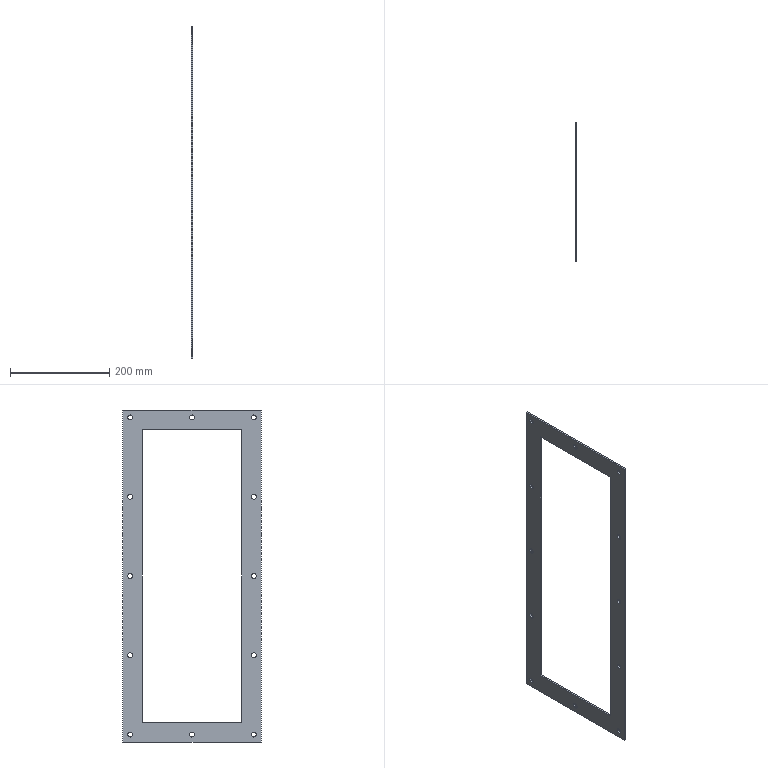Part | SolidWorks | features ExtruThin 1, HoleWzd 1, LPattern 1 | 1 solid | 34 faces | box 4 x 280 x 670 mm | volume 274630 mm3 | cylinder 24 | plane 10 | commonest cylinder face diameters 10 x24
STEP:
#1=CARTESIAN_POINT('',(0.,-125.,-315.));
#2=VERTEX_POINT('',#1);
#3=CARTESIAN_POINT('',(0.,-125.,-325.));
#4=VERTEX_POINT('',#3);
#5=CARTESIAN_POINT('',(0.,-125.,-320.));
#6=DIRECTION('',(1.,0.,0.));
#7=DIRECTION('',(0.,0.,-1.));
#8=AXIS2_PLACEMENT_3D('',#5,#6,#7);
#9=CIRCLE('',#8,5.);
#10=EDGE_CURVE('',#2,#4,#9,.T.);
#11=ORIENTED_EDGE('',*,*,#10,.F.);
#12=CARTESIAN_POINT('',(4.,-125.,-315.));
#13=VERTEX_POINT('',#12);
#14=CARTESIAN_POINT('',(4.,-125.,-315.));
#15=DIRECTION('',(1.,0.,0.));
#16=VECTOR('',#15,1000.);
#17=LINE('',#14,#16);
#18=EDGE_CURVE('',#2,#13,#17,.T.);
#19=ORIENTED_EDGE('',*,*,#18,.T.);
#20=CARTESIAN_POINT('',(4.,-125.,-325.));
#21=VERTEX_POINT('',#20);
#22=CARTESIAN_POINT('',(4.,-125.,-320.));
#23=DIRECTION('',(1.,0.,0.));
#24=DIRECTION('',(0.,0.,-1.));
#25=AXIS2_PLACEMENT_3D('',#22,#23,#24);
#26=CIRCLE('',#25,5.);
#27=EDGE_CURVE('',#13,#21,#26,.T.);
#28=ORIENTED_EDGE('',*,*,#27,.T.);
#29=CARTESIAN_POINT('',(4.,-125.,-325.));
#30=DIRECTION('',(1.,0.,0.));
#31=VECTOR('',#30,1000.);
#32=LINE('',#29,#31);
#33=EDGE_CURVE('',#4,#21,#32,.T.);
#34=ORIENTED_EDGE('',*,*,#33,.F.);
#35=EDGE_LOOP('',(#11,#19,#28,#34));
#36=FACE_OUTER_BOUND('',#35,.T.);
#37=CARTESIAN_POINT('',(4.,-125.,-320.));
#38=DIRECTION('',(1.,0.,0.));
#39=DIRECTION('',(0.,0.,-1.));
#40=AXIS2_PLACEMENT_3D('',#37,#38,#39);
#41=CYLINDRICAL_SURFACE('',#40,5.);
#42=ADVANCED_FACE('',(#36),#41,.F.);
#43=CARTESIAN_POINT('',(0.,0.,-315.));
#44=VERTEX_POINT('',#43);
#45=CARTESIAN_POINT('',(0.,0.,-325.));
#46=VERTEX_POINT('',#45);
#47=CARTESIAN_POINT('',(0.,0.,-320.));
#48=DIRECTION('',(1.,0.,0.));
#49=DIRECTION('',(0.,0.,-1.));
#50=AXIS2_PLACEMENT_3D('',#47,#48,#49);
#51=CIRCLE('',#50,5.);
#52=EDGE_CURVE('',#44,#46,#51,.T.);
#53=ORIENTED_EDGE('',*,*,#52,.F.);
#54=CARTESIAN_POINT('',(4.,0.,-315.));
#55=VERTEX_POINT('',#54);
#56=CARTESIAN_POINT('',(4.,0.,-315.));
#57=DIRECTION('',(1.,0.,0.));
#58=VECTOR('',#57,1000.);
#59=LINE('',#56,#58);
#60=EDGE_CURVE('',#44,#55,#59,.T.);
#61=ORIENTED_EDGE('',*,*,#60,.T.);
#62=CARTESIAN_POINT('',(4.,0.,-325.));
#63=VERTEX_POINT('',#62);
#64=CARTESIAN_POINT('',(4.,0.,-320.));
#65=DIRECTION('',(1.,0.,0.));
#66=DIRECTION('',(0.,0.,-1.));
#67=AXIS2_PLACEMENT_3D('',#64,#65,#66);
#68=CIRCLE('',#67,5.);
#69=EDGE_CURVE('',#55,#63,#68,.T.);
#70=ORIENTED_EDGE('',*,*,#69,.T.);
#71=CARTESIAN_POINT('',(4.,0.,-325.));
#72=DIRECTION('',(1.,0.,0.));
#73=VECTOR('',#72,1000.);
#74=LINE('',#71,#73);
#75=EDGE_CURVE('',#46,#63,#74,.T.);
#76=ORIENTED_EDGE('',*,*,#75,.F.);
#77=EDGE_LOOP('',(#53,#61,#70,#76));
#78=FACE_OUTER_BOUND('',#77,.T.);
#79=CARTESIAN_POINT('',(4.,0.,-320.));
#80=DIRECTION('',(1.,0.,0.));
#81=DIRECTION('',(0.,0.,-1.));
#82=AXIS2_PLACEMENT_3D('',#79,#80,#81);
#83=CYLINDRICAL_SURFACE('',#82,5.);
#84=ADVANCED_FACE('',(#78),#83,.F.);
#85=CARTESIAN_POINT('',(0.,125.,-315.));
#86=VERTEX_POINT('',#85);
#87=CARTESIAN_POINT('',(0.,125.,-325.));
#88=VERTEX_POINT('',#87);
#89=CARTESIAN_POINT('',(0.,125.,-320.));
#90=DIRECTION('',(1.,0.,0.));
#91=DIRECTION('',(0.,0.,-1.));
#92=AXIS2_PLACEMENT_3D('',#89,#90,#91);
#93=CIRCLE('',#92,5.);
#94=EDGE_CURVE('',#86,#88,#93,.T.);
#95=ORIENTED_EDGE('',*,*,#94,.F.);
#96=CARTESIAN_POINT('',(4.,125.,-315.));
#97=VERTEX_POINT('',#96);
#98=CARTESIAN_POINT('',(4.,125.,-315.));
#99=DIRECTION('',(1.,0.,0.));
#100=VECTOR('',#99,1000.);
#101=LINE('',#98,#100);
#102=EDGE_CURVE('',#86,#97,#101,.T.);
#103=ORIENTED_EDGE('',*,*,#102,.T.);
#104=CARTESIAN_POINT('',(4.,125.,-325.));
#105=VERTEX_POINT('',#104);
#106=CARTESIAN_POINT('',(4.,125.,-320.));
#107=DIRECTION('',(1.,0.,0.));
#108=DIRECTION('',(0.,0.,-1.));
#109=AXIS2_PLACEMENT_3D('',#106,#107,#108);
#110=CIRCLE('',#109,5.);
#111=EDGE_CURVE('',#97,#105,#110,.T.);
#112=ORIENTED_EDGE('',*,*,#111,.T.);
#113=CARTESIAN_POINT('',(4.,125.,-325.));
#114=DIRECTION('',(1.,0.,0.));
#115=VECTOR('',#114,1000.);
#116=LINE('',#113,#115);
#117=EDGE_CURVE('',#88,#105,#116,.T.);
#118=ORIENTED_EDGE('',*,*,#117,.F.);
#119=EDGE_LOOP('',(#95,#103,#112,#118));
#120=FACE_OUTER_BOUND('',#119,.T.);
#121=CARTESIAN_POINT('',(4.,125.,-320.));
#122=DIRECTION('',(1.,0.,0.));
#123=DIRECTION('',(0.,0.,-1.));
#124=AXIS2_PLACEMENT_3D('',#121,#122,#123);
#125=CYLINDRICAL_SURFACE('',#124,5.);
#126=ADVANCED_FACE('',(#120),#125,.F.);
#127=CARTESIAN_POINT('',(0.,-125.,-155.));
#128=VERTEX_POINT('',#127);
#129=CARTESIAN_POINT('',(0.,-125.,-165.));
#130=VERTEX_POINT('',#129);
#131=CARTESIAN_POINT('',(0.,-125.,-160.));
#132=DIRECTION('',(1.,0.,0.));
#133=DIRECTION('',(0.,0.,-1.));
#134=AXIS2_PLACEMENT_3D('',#131,#132,#133);
#135=CIRCLE('',#134,5.);
#136=EDGE_CURVE('',#128,#130,#135,.T.);
#137=ORIENTED_EDGE('',*,*,#136,.F.);
#138=CARTESIAN_POINT('',(4.,-125.,-155.));
#139=VERTEX_POINT('',#138);
#140=CARTESIAN_POINT('',(4.,-125.,-155.));
#141=DIRECTION('',(1.,0.,0.));
#142=VECTOR('',#141,1000.);
#143=LINE('',#140,#142);
#144=EDGE_CURVE('',#128,#139,#143,.T.);
#145=ORIENTED_EDGE('',*,*,#144,.T.);
#146=CARTESIAN_POINT('',(4.,-125.,-165.));
#147=VERTEX_POINT('',#146);
#148=CARTESIAN_POINT('',(4.,-125.,-160.));
#149=DIRECTION('',(1.,0.,0.));
#150=DIRECTION('',(0.,0.,-1.));
#151=AXIS2_PLACEMENT_3D('',#148,#149,#150);
#152=CIRCLE('',#151,5.);
#153=EDGE_CURVE('',#139,#147,#152,.T.);
#154=ORIENTED_EDGE('',*,*,#153,.T.);
#155=CARTESIAN_POINT('',(4.,-125.,-165.));
#156=DIRECTION('',(1.,0.,0.));
#157=VECTOR('',#156,1000.);
#158=LINE('',#155,#157);
#159=EDGE_CURVE('',#130,#147,#158,.T.);
#160=ORIENTED_EDGE('',*,*,#159,.F.);
#161=EDGE_LOOP('',(#137,#145,#154,#160));
#162=FACE_OUTER_BOUND('',#161,.T.);
#163=CARTESIAN_POINT('',(4.,-125.,-160.));
#164=DIRECTION('',(1.,0.,0.));
#165=DIRECTION('',(0.,0.,-1.));
#166=AXIS2_PLACEMENT_3D('',#163,#164,#165);
#167=CYLINDRICAL_SURFACE('',#166,5.);
#168=ADVANCED_FACE('',(#162),#167,.F.);
#169=CARTESIAN_POINT('',(0.,125.,-155.));
#170=VERTEX_POINT('',#169);
#171=CARTESIAN_POINT('',(0.,125.,-165.));
#172=VERTEX_POINT('',#171);
#173=CARTESIAN_POINT('',(0.,125.,-160.));
#174=DIRECTION('',(1.,0.,0.));
#175=DIRECTION('',(0.,0.,-1.));
#176=AXIS2_PLACEMENT_3D('',#173,#174,#175);
#177=CIRCLE('',#176,5.);
#178=EDGE_CURVE('',#170,#172,#177,.T.);
#179=ORIENTED_EDGE('',*,*,#178,.F.);
#180=CARTESIAN_POINT('',(4.,125.,-155.));
#181=VERTEX_POINT('',#180);
#182=CARTESIAN_POINT('',(4.,125.,-155.));
#183=DIRECTION('',(1.,0.,0.));
#184=VECTOR('',#183,1000.);
#185=LINE('',#182,#184);
#186=EDGE_CURVE('',#170,#181,#185,.T.);
#187=ORIENTED_EDGE('',*,*,#186,.T.);
#188=CARTESIAN_POINT('',(4.,125.,-165.));
#189=VERTEX_POINT('',#188);
#190=CARTESIAN_POINT('',(4.,125.,-160.));
#191=DIRECTION('',(1.,0.,0.));
#192=DIRECTION('',(0.,0.,-1.));
#193=AXIS2_PLACEMENT_3D('',#190,#191,#192);
#194=CIRCLE('',#193,5.);
#195=EDGE_CURVE('',#181,#189,#194,.T.);
#196=ORIENTED_EDGE('',*,*,#195,.T.);
#197=CARTESIAN_POINT('',(4.,125.,-165.));
#198=DIRECTION('',(1.,0.,0.));
#199=VECTOR('',#198,1000.);
#200=LINE('',#197,#199);
#201=EDGE_CURVE('',#172,#189,#200,.T.);
#202=ORIENTED_EDGE('',*,*,#201,.F.);
#203=EDGE_LOOP('',(#179,#187,#196,#202));
#204=FACE_OUTER_BOUND('',#203,.T.);
#205=CARTESIAN_POINT('',(4.,125.,-160.));
#206=DIRECTION('',(1.,0.,0.));
#207=DIRECTION('',(0.,0.,-1.));
#208=AXIS2_PLACEMENT_3D('',#205,#206,#207);
#209=CYLINDRICAL_SURFACE('',#208,5.);
#210=ADVANCED_FACE('',(#204),#209,.F.);
#211=CARTESIAN_POINT('',(0.,-125.,5.));
#212=VERTEX_POINT('',#211);
#213=CARTESIAN_POINT('',(0.,-125.,-5.));
#214=VERTEX_POINT('',#213);
#215=CARTESIAN_POINT('',(0.,-125.,0.));
#216=DIRECTION('',(1.,0.,0.));
#217=DIRECTION('',(0.,0.,-1.));
#218=AXIS2_PLACEMENT_3D('',#215,#216,#217);
#219=CIRCLE('',#218,5.);
#220=EDGE_CURVE('',#212,#214,#219,.T.);
#221=ORIENTED_EDGE('',*,*,#220,.F.);
#222=CARTESIAN_POINT('',(4.,-125.,5.));
#223=VERTEX_POINT('',#222);
#224=CARTESIAN_POINT('',(4.,-125.,5.));
#225=DIRECTION('',(1.,0.,0.));
#226=VECTOR('',#225,1000.);
#227=LINE('',#224,#226);
#228=EDGE_CURVE('',#212,#223,#227,.T.);
#229=ORIENTED_EDGE('',*,*,#228,.T.);
#230=CARTESIAN_POINT('',(4.,-125.,-5.));
#231=VERTEX_POINT('',#230);
#232=CARTESIAN_POINT('',(4.,-125.,0.));
#233=DIRECTION('',(1.,0.,0.));
#234=DIRECTION('',(0.,0.,-1.));
#235=AXIS2_PLACEMENT_3D('',#232,#233,#234);
#236=CIRCLE('',#235,5.);
#237=EDGE_CURVE('',#223,#231,#236,.T.);
#238=ORIENTED_EDGE('',*,*,#237,.T.);
#239=CARTESIAN_POINT('',(4.,-125.,-5.));
#240=DIRECTION('',(1.,0.,0.));
#241=VECTOR('',#240,1000.);
#242=LINE('',#239,#241);
#243=EDGE_CURVE('',#214,#231,#242,.T.);
#244=ORIENTED_EDGE('',*,*,#243,.F.);
#245=EDGE_LOOP('',(#221,#229,#238,#244));
#246=FACE_OUTER_BOUND('',#245,.T.);
#247=CARTESIAN_POINT('',(4.,-125.,0.));
#248=DIRECTION('',(1.,0.,0.));
#249=DIRECTION('',(0.,0.,-1.));
#250=AXIS2_PLACEMENT_3D('',#247,#248,#249);
#251=CYLINDRICAL_SURFACE('',#250,5.);
#252=ADVANCED_FACE('',(#246),#251,.F.);
#253=CARTESIAN_POINT('',(0.,125.,5.));
#254=VERTEX_POINT('',#253);
#255=CARTESIAN_POINT('',(0.,125.,-5.));
#256=VERTEX_POINT('',#255);
#257=CARTESIAN_POINT('',(0.,125.,0.));
#258=DIRECTION('',(1.,0.,0.));
#259=DIRECTION('',(0.,0.,-1.));
#260=AXIS2_PLACEMENT_3D('',#257,#258,#259);
#261=CIRCLE('',#260,5.);
#262=EDGE_CURVE('',#254,#256,#261,.T.);
#263=ORIENTED_EDGE('',*,*,#262,.F.);
#264=CARTESIAN_POINT('',(4.,125.,5.));
#265=VERTEX_POINT('',#264);
#266=CARTESIAN_POINT('',(4.,125.,5.));
#267=DIRECTION('',(1.,0.,0.));
#268=VECTOR('',#267,1000.);
#269=LINE('',#266,#268);
#270=EDGE_CURVE('',#254,#265,#269,.T.);
#271=ORIENTED_EDGE('',*,*,#270,.T.);
#272=CARTESIAN_POINT('',(4.,125.,-5.));
#273=VERTEX_POINT('',#272);
#274=CARTESIAN_POINT('',(4.,125.,0.));
#275=DIRECTION('',(1.,0.,0.));
#276=DIRECTION('',(0.,0.,-1.));
#277=AXIS2_PLACEMENT_3D('',#274,#275,#276);
#278=CIRCLE('',#277,5.);
#279=EDGE_CURVE('',#265,#273,#278,.T.);
#280=ORIENTED_EDGE('',*,*,#279,.T.);
#281=CARTESIAN_POINT('',(4.,125.,-5.));
#282=DIRECTION('',(1.,0.,0.));
#283=VECTOR('',#282,1000.);
#284=LINE('',#281,#283);
#285=EDGE_CURVE('',#256,#273,#284,.T.);
#286=ORIENTED_EDGE('',*,*,#285,.F.);
#287=EDGE_LOOP('',(#263,#271,#280,#286));
#288=FACE_OUTER_BOUND('',#287,.T.);
#289=CARTESIAN_POINT('',(4.,125.,0.));
#290=DIRECTION('',(1.,0.,0.));
#291=DIRECTION('',(0.,0.,-1.));
#292=AXIS2_PLACEMENT_3D('',#289,#290,#291);
#293=CYLINDRICAL_SURFACE('',#292,5.);
#294=ADVANCED_FACE('',(#288),#293,.F.);
#295=CARTESIAN_POINT('',(0.,-125.,165.));
#296=VERTEX_POINT('',#295);
#297=CARTESIAN_POINT('',(0.,-125.,155.));
#298=VERTEX_POINT('',#297);
#299=CARTESIAN_POINT('',(0.,-125.,160.));
#300=DIRECTION('',(1.,0.,0.));
#301=DIRECTION('',(0.,0.,-1.));
#302=AXIS2_PLACEMENT_3D('',#299,#300,#301);
#303=CIRCLE('',#302,5.);
#304=EDGE_CURVE('',#296,#298,#303,.T.);
#305=ORIENTED_EDGE('',*,*,#304,.F.);
#306=CARTESIAN_POINT('',(4.,-125.,165.));
#307=VERTEX_POINT('',#306);
#308=CARTESIAN_POINT('',(4.,-125.,165.));
#309=DIRECTION('',(1.,0.,0.));
#310=VECTOR('',#309,1000.);
#311=LINE('',#308,#310);
#312=EDGE_CURVE('',#296,#307,#311,.T.);
#313=ORIENTED_EDGE('',*,*,#312,.T.);
#314=CARTESIAN_POINT('',(4.,-125.,155.));
#315=VERTEX_POINT('',#314);
#316=CARTESIAN_POINT('',(4.,-125.,160.));
#317=DIRECTION('',(1.,0.,0.));
#318=DIRECTION('',(0.,0.,-1.));
#319=AXIS2_PLACEMENT_3D('',#316,#317,#318);
#320=CIRCLE('',#319,5.);
#321=EDGE_CURVE('',#307,#315,#320,.T.);
#322=ORIENTED_EDGE('',*,*,#321,.T.);
#323=CARTESIAN_POINT('',(4.,-125.,155.));
#324=DIRECTION('',(1.,0.,0.));
#325=VECTOR('',#324,1000.);
#326=LINE('',#323,#325);
#327=EDGE_CURVE('',#298,#315,#326,.T.);
#328=ORIENTED_EDGE('',*,*,#327,.F.);
#329=EDGE_LOOP('',(#305,#313,#322,#328));
#330=FACE_OUTER_BOUND('',#329,.T.);
#331=CARTESIAN_POINT('',(4.,-125.,160.));
#332=DIRECTION('',(1.,0.,0.));
#333=DIRECTION('',(0.,0.,-1.));
#334=AXIS2_PLACEMENT_3D('',#331,#332,#333);
#335=CYLINDRICAL_SURFACE('',#334,5.);
#336=ADVANCED_FACE('',(#330),#335,.F.);
#337=CARTESIAN_POINT('',(0.,125.,165.));
#338=VERTEX_POINT('',#337);
#339=CARTESIAN_POINT('',(0.,125.,155.));
#340=VERTEX_POINT('',#339);
#341=CARTESIAN_POINT('',(0.,125.,160.));
#342=DIRECTION('',(1.,0.,0.));
#343=DIRECTION('',(0.,0.,-1.));
#344=AXIS2_PLACEMENT_3D('',#341,#342,#343);
#345=CIRCLE('',#344,5.);
#346=EDGE_CURVE('',#338,#340,#345,.T.);
#347=ORIENTED_EDGE('',*,*,#346,.F.);
#348=CARTESIAN_POINT('',(4.,125.,165.));
#349=VERTEX_POINT('',#348);
#350=CARTESIAN_POINT('',(4.,125.,165.));
#351=DIRECTION('',(1.,0.,0.));
#352=VECTOR('',#351,1000.);
#353=LINE('',#350,#352);
#354=EDGE_CURVE('',#338,#349,#353,.T.);
#355=ORIENTED_EDGE('',*,*,#354,.T.);
#356=CARTESIAN_POINT('',(4.,125.,155.));
#357=VERTEX_POINT('',#356);
#358=CARTESIAN_POINT('',(4.,125.,160.));
#359=DIRECTION('',(1.,0.,0.));
#360=DIRECTION('',(0.,0.,-1.));
#361=AXIS2_PLACEMENT_3D('',#358,#359,#360);
#362=CIRCLE('',#361,5.);
#363=EDGE_CURVE('',#349,#357,#362,.T.);
#364=ORIENTED_EDGE('',*,*,#363,.T.);
#365=CARTESIAN_POINT('',(4.,125.,155.));
#366=DIRECTION('',(1.,0.,0.));
#367=VECTOR('',#366,1000.);
#368=LINE('',#365,#367);
#369=EDGE_CURVE('',#340,#357,#368,.T.);
#370=ORIENTED_EDGE('',*,*,#369,.F.);
#371=EDGE_LOOP('',(#347,#355,#364,#370));
#372=FACE_OUTER_BOUND('',#371,.T.);
#373=CARTESIAN_POINT('',(4.,125.,160.));
#374=DIRECTION('',(1.,0.,0.));
#375=DIRECTION('',(0.,0.,-1.));
#376=AXIS2_PLACEMENT_3D('',#373,#374,#375);
#377=CYLINDRICAL_SURFACE('',#376,5.);
#378=ADVANCED_FACE('',(#372),#377,.F.);
#379=CARTESIAN_POINT('',(0.,-125.,325.));
#380=VERTEX_POINT('',#379);
#381=CARTESIAN_POINT('',(0.,-125.,315.));
#382=VERTEX_POINT('',#381);
#383=CARTESIAN_POINT('',(0.,-125.,320.));
#384=DIRECTION('',(1.,0.,0.));
#385=DIRECTION('',(0.,0.,-1.));
#386=AXIS2_PLACEMENT_3D('',#383,#384,#385);
#387=CIRCLE('',#386,5.);
#388=EDGE_CURVE('',#380,#382,#387,.T.);
#389=ORIENTED_EDGE('',*,*,#388,.F.);
#390=CARTESIAN_POINT('',(4.,-125.,325.));
#391=VERTEX_POINT('',#390);
#392=CARTESIAN_POINT('',(4.,-125.,325.));
#393=DIRECTION('',(1.,0.,0.));
#394=VECTOR('',#393,1000.);
#395=LINE('',#392,#394);
#396=EDGE_CURVE('',#380,#391,#395,.T.);
#397=ORIENTED_EDGE('',*,*,#396,.T.);
#398=CARTESIAN_POINT('',(4.,-125.,315.));
#399=VERTEX_POINT('',#398);
#400=CARTESIAN_POINT('',(4.,-125.,320.));
#401=DIRECTION('',(1.,0.,0.));
#402=DIRECTION('',(0.,0.,-1.));
#403=AXIS2_PLACEMENT_3D('',#400,#401,#402);
#404=CIRCLE('',#403,5.);
#405=EDGE_CURVE('',#391,#399,#404,.T.);
#406=ORIENTED_EDGE('',*,*,#405,.T.);
#407=CARTESIAN_POINT('',(4.,-125.,315.));
#408=DIRECTION('',(1.,0.,0.));
#409=VECTOR('',#408,1000.);
#410=LINE('',#407,#409);
#411=EDGE_CURVE('',#382,#399,#410,.T.);
#412=ORIENTED_EDGE('',*,*,#411,.F.);
#413=EDGE_LOOP('',(#389,#397,#406,#412));
#414=FACE_OUTER_BOUND('',#413,.T.);
#415=CARTESIAN_POINT('',(4.,-125.,320.));
#416=DIRECTION('',(1.,0.,0.));
#417=DIRECTION('',(0.,0.,-1.));
#418=AXIS2_PLACEMENT_3D('',#415,#416,#417);
#419=CYLINDRICAL_SURFACE('',#418,5.);
#420=ADVANCED_FACE('',(#414),#419,.F.);
#421=CARTESIAN_POINT('',(0.,0.,325.));
#422=VERTEX_POINT('',#421);
#423=CARTESIAN_POINT('',(0.,0.,315.));
#424=VERTEX_POINT('',#423);
#425=CARTESIAN_POINT('',(0.,0.,320.));
#426=DIRECTION('',(1.,0.,0.));
#427=DIRECTION('',(0.,0.,-1.));
#428=AXIS2_PLACEMENT_3D('',#425,#426,#427);
#429=CIRCLE('',#428,5.);
#430=EDGE_CURVE('',#422,#424,#429,.T.);
#431=ORIENTED_EDGE('',*,*,#430,.F.);
#432=CARTESIAN_POINT('',(4.,0.,325.));
#433=VERTEX_POINT('',#432);
#434=CARTESIAN_POINT('',(4.,0.,325.));
#435=DIRECTION('',(1.,0.,0.));
#436=VECTOR('',#435,1000.);
#437=LINE('',#434,#436);
#438=EDGE_CURVE('',#422,#433,#437,.T.);
#439=ORIENTED_EDGE('',*,*,#438,.T.);
#440=CARTESIAN_POINT('',(4.,0.,315.));
#441=VERTEX_POINT('',#440);
#442=CARTESIAN_POINT('',(4.,0.,320.));
#443=DIRECTION('',(1.,0.,0.));
#444=DIRECTION('',(0.,0.,-1.));
#445=AXIS2_PLACEMENT_3D('',#442,#443,#444);
#446=CIRCLE('',#445,5.);
#447=EDGE_CURVE('',#433,#441,#446,.T.);
#448=ORIENTED_EDGE('',*,*,#447,.T.);
#449=CARTESIAN_POINT('',(4.,0.,315.));
#450=DIRECTION('',(1.,0.,0.));
#451=VECTOR('',#450,1000.);
#452=LINE('',#449,#451);
#453=EDGE_CURVE('',#424,#441,#452,.T.);
#454=ORIENTED_EDGE('',*,*,#453,.F.);
#455=EDGE_LOOP('',(#431,#439,#448,#454));
#456=FACE_OUTER_BOUND('',#455,.T.);
#457=CARTESIAN_POINT('',(4.,0.,320.));
#458=DIRECTION('',(1.,0.,0.));
#459=DIRECTION('',(0.,0.,-1.));
#460=AXIS2_PLACEMENT_3D('',#457,#458,#459);
#461=CYLINDRICAL_SURFACE('',#460,5.);
#462=ADVANCED_FACE('',(#456),#461,.F.);
#463=CARTESIAN_POINT('',(0.,125.,325.));
#464=VERTEX_POINT('',#463);
#465=CARTESIAN_POINT('',(0.,125.,315.));
#466=VERTEX_POINT('',#465);
#467=CARTESIAN_POINT('',(0.,125.,320.));
#468=DIRECTION('',(1.,0.,0.));
#469=DIRECTION('',(0.,0.,-1.));
#470=AXIS2_PLACEMENT_3D('',#467,#468,#469);
#471=CIRCLE('',#470,5.);
#472=EDGE_CURVE('',#464,#466,#471,.T.);
#473=ORIENTED_EDGE('',*,*,#472,.F.);
#474=CARTESIAN_POINT('',(4.,125.,325.));
#475=VERTEX_POINT('',#474);
#476=CARTESIAN_POINT('',(4.,125.,325.));
#477=DIRECTION('',(1.,0.,0.));
#478=VECTOR('',#477,1000.);
#479=LINE('',#476,#478);
#480=EDGE_CURVE('',#464,#475,#479,.T.);
#481=ORIENTED_EDGE('',*,*,#480,.T.);
#482=CARTESIAN_POINT('',(4.,125.,315.));
#483=VERTEX_POINT('',#482);
#484=CARTESIAN_POINT('',(4.,125.,320.));
#485=DIRECTION('',(1.,0.,0.));
#486=DIRECTION('',(0.,0.,-1.));
#487=AXIS2_PLACEMENT_3D('',#484,#485,#486);
#488=CIRCLE('',#487,5.);
#489=EDGE_CURVE('',#475,#483,#488,.T.);
#490=ORIENTED_EDGE('',*,*,#489,.T.);
#491=CARTESIAN_POINT('',(4.,125.,315.));
#492=DIRECTION('',(1.,0.,0.));
#493=VECTOR('',#492,1000.);
#494=LINE('',#491,#493);
#495=EDGE_CURVE('',#466,#483,#494,.T.);
#496=ORIENTED_EDGE('',*,*,#495,.F.);
#497=EDGE_LOOP('',(#473,#481,#490,#496));
#498=FACE_OUTER_BOUND('',#497,.T.);
#499=CARTESIAN_POINT('',(4.,125.,320.));
#500=DIRECTION('',(1.,0.,0.));
#501=DIRECTION('',(0.,0.,-1.));
#502=AXIS2_PLACEMENT_3D('',#499,#500,#501);
#503=CYLINDRICAL_SURFACE('',#502,5.);
#504=ADVANCED_FACE('',(#498),#503,.F.);
#505=CARTESIAN_POINT('',(4.,-125.,-320.));
#506=DIRECTION('',(1.,0.,0.));
#507=DIRECTION('',(0.,0.,-1.));
#508=AXIS2_PLACEMENT_3D('',#505,#506,#507);
#509=CIRCLE('',#508,5.);
#510=EDGE_CURVE('',#21,#13,#509,.T.);
#511=ORIENTED_EDGE('',*,*,#510,.F.);
#512=ORIENTED_EDGE('',*,*,#27,.F.);
#513=EDGE_LOOP('',(#511,#512));
#514=FACE_BOUND('',#513,.T.);
#515=CARTESIAN_POINT('',(4.,0.,-320.));
#516=DIRECTION('',(1.,0.,0.));
#517=DIRECTION('',(0.,0.,-1.));
#518=AXIS2_PLACEMENT_3D('',#515,#516,#517);
#519=CIRCLE('',#518,5.);
#520=EDGE_CURVE('',#63,#55,#519,.T.);
#521=ORIENTED_EDGE('',*,*,#520,.F.);
#522=ORIENTED_EDGE('',*,*,#69,.F.);
#523=EDGE_LOOP('',(#521,#522));
#524=FACE_BOUND('',#523,.T.);
#525=CARTESIAN_POINT('',(4.,125.,-320.));
#526=DIRECTION('',(1.,0.,0.));
#527=DIRECTION('',(0.,0.,-1.));
#528=AXIS2_PLACEMENT_3D('',#525,#526,#527);
#529=CIRCLE('',#528,5.);
#530=EDGE_CURVE('',#105,#97,#529,.T.);
#531=ORIENTED_EDGE('',*,*,#530,.F.);
#532=ORIENTED_EDGE('',*,*,#111,.F.);
#533=EDGE_LOOP('',(#531,#532));
#534=FACE_BOUND('',#533,.T.);
#535=CARTESIAN_POINT('',(4.,-125.,-160.));
#536=DIRECTION('',(1.,0.,0.));
#537=DIRECTION('',(0.,0.,-1.));
#538=AXIS2_PLACEMENT_3D('',#535,#536,#537);
#539=CIRCLE('',#538,5.);
#540=EDGE_CURVE('',#147,#139,#539,.T.);
#541=ORIENTED_EDGE('',*,*,#540,.F.);
#542=ORIENTED_EDGE('',*,*,#153,.F.);
#543=EDGE_LOOP('',(#541,#542));
#544=FACE_BOUND('',#543,.T.);
#545=CARTESIAN_POINT('',(4.,125.,-160.));
#546=DIRECTION('',(1.,0.,0.));
#547=DIRECTION('',(0.,0.,-1.));
#548=AXIS2_PLACEMENT_3D('',#545,#546,#547);
#549=CIRCLE('',#548,5.);
#550=EDGE_CURVE('',#189,#181,#549,.T.);
#551=ORIENTED_EDGE('',*,*,#550,.F.);
#552=ORIENTED_EDGE('',*,*,#195,.F.);
#553=EDGE_LOOP('',(#551,#552));
#554=FACE_BOUND('',#553,.T.);
#555=CARTESIAN_POINT('',(4.,-125.,0.));
#556=DIRECTION('',(1.,0.,0.));
#557=DIRECTION('',(0.,0.,-1.));
#558=AXIS2_PLACEMENT_3D('',#555,#556,#557);
#559=CIRCLE('',#558,5.);
#560=EDGE_CURVE('',#231,#223,#559,.T.);
#561=ORIENTED_EDGE('',*,*,#560,.F.);
#562=ORIENTED_EDGE('',*,*,#237,.F.);
#563=EDGE_LOOP('',(#561,#562));
#564=FACE_BOUND('',#563,.T.);
#565=CARTESIAN_POINT('',(4.,125.,0.));
#566=DIRECTION('',(1.,0.,0.));
#567=DIRECTION('',(0.,0.,-1.));
#568=AXIS2_PLACEMENT_3D('',#565,#566,#567);
#569=CIRCLE('',#568,5.);
#570=EDGE_CURVE('',#273,#265,#569,.T.);
#571=ORIENTED_EDGE('',*,*,#570,.F.);
#572=ORIENTED_EDGE('',*,*,#279,.F.);
#573=EDGE_LOOP('',(#571,#572));
#574=FACE_BOUND('',#573,.T.);
#575=CARTESIAN_POINT('',(4.,-125.,160.));
#576=DIRECTION('',(1.,0.,0.));
#577=DIRECTION('',(0.,0.,-1.));
#578=AXIS2_PLACEMENT_3D('',#575,#576,#577);
#579=CIRCLE('',#578,5.);
#580=EDGE_CURVE('',#315,#307,#579,.T.);
#581=ORIENTED_EDGE('',*,*,#580,.F.);
#582=ORIENTED_EDGE('',*,*,#321,.F.);
#583=EDGE_LOOP('',(#581,#582));
#584=FACE_BOUND('',#583,.T.);
#585=CARTESIAN_POINT('',(4.,125.,160.));
#586=DIRECTION('',(1.,0.,0.));
#587=DIRECTION('',(0.,0.,-1.));
#588=AXIS2_PLACEMENT_3D('',#585,#586,#587);
#589=CIRCLE('',#588,5.);
#590=EDGE_CURVE('',#357,#349,#589,.T.);
#591=ORIENTED_EDGE('',*,*,#590,.F.);
#592=ORIENTED_EDGE('',*,*,#363,.F.);
#593=EDGE_LOOP('',(#591,#592));
#594=FACE_BOUND('',#593,.T.);
#595=CARTESIAN_POINT('',(4.,-125.,320.));
#596=DIRECTION('',(1.,0.,0.));
#597=DIRECTION('',(0.,0.,-1.));
#598=AXIS2_PLACEMENT_3D('',#595,#596,#597);
#599=CIRCLE('',#598,5.);
#600=EDGE_CURVE('',#399,#391,#599,.T.);
#601=ORIENTED_EDGE('',*,*,#600,.F.);
#602=ORIENTED_EDGE('',*,*,#405,.F.);
#603=EDGE_LOOP('',(#601,#602));
#604=FACE_BOUND('',#603,.T.);
#605=CARTESIAN_POINT('',(4.,0.,320.));
#606=DIRECTION('',(1.,0.,0.));
#607=DIRECTION('',(0.,0.,-1.));
#608=AXIS2_PLACEMENT_3D('',#605,#606,#607);
#609=CIRCLE('',#608,5.);
#610=EDGE_CURVE('',#441,#433,#609,.T.);
#611=ORIENTED_EDGE('',*,*,#610,.F.);
#612=ORIENTED_EDGE('',*,*,#447,.F.);
#613=EDGE_LOOP('',(#611,#612));
#614=FACE_BOUND('',#613,.T.);
#615=CARTESIAN_POINT('',(4.,125.,320.));
#616=DIRECTION('',(1.,0.,0.));
#617=DIRECTION('',(0.,0.,-1.));
#618=AXIS2_PLACEMENT_3D('',#615,#616,#617);
#619=CIRCLE('',#618,5.);
#620=EDGE_CURVE('',#483,#475,#619,.T.);
#621=ORIENTED_EDGE('',*,*,#620,.F.);
#622=ORIENTED_EDGE('',*,*,#489,.F.);
#623=EDGE_LOOP('',(#621,#622));
#624=FACE_BOUND('',#623,.T.);
#625=CARTESIAN_POINT('',(4.,140.,335.));
#626=VERTEX_POINT('',#625);
#627=CARTESIAN_POINT('',(4.,-140.,335.));
#628=VERTEX_POINT('',#627);
#629=CARTESIAN_POINT('',(4.,140.,335.));
#630=DIRECTION('',(0.,-1.,0.));
#631=VECTOR('',#630,1000.);
#632=LINE('',#629,#631);
#633=EDGE_CURVE('',#626,#628,#632,.T.);
#634=ORIENTED_EDGE('',*,*,#633,.T.);
#635=CARTESIAN_POINT('',(4.,-140.,-335.));
#636=VERTEX_POINT('',#635);
#637=CARTESIAN_POINT('',(4.,-140.,335.));
#638=DIRECTION('',(0.,0.,-1.));
#639=VECTOR('',#638,1000.);
#640=LINE('',#637,#639);
#641=EDGE_CURVE('',#628,#636,#640,.T.);
#642=ORIENTED_EDGE('',*,*,#641,.T.);
#643=CARTESIAN_POINT('',(4.,140.,-335.));
#644=VERTEX_POINT('',#643);
#645=CARTESIAN_POINT('',(4.,140.,-335.));
#646=DIRECTION('',(0.,1.,0.));
#647=VECTOR('',#646,1000.);
#648=LINE('',#645,#647);
#649=EDGE_CURVE('',#636,#644,#648,.T.);
#650=ORIENTED_EDGE('',*,*,#649,.T.);
#651=CARTESIAN_POINT('',(4.,140.,335.));
#652=DIRECTION('',(0.,0.,1.));
#653=VECTOR('',#652,1000.);
#654=LINE('',#651,#653);
#655=EDGE_CURVE('',#644,#626,#654,.T.);
#656=ORIENTED_EDGE('',*,*,#655,.T.);
#657=EDGE_LOOP('',(#634,#642,#650,#656));
#658=FACE_OUTER_BOUND('',#657,.T.);
#659=CARTESIAN_POINT('',(4.,-100.,295.));
#660=VERTEX_POINT('',#659);
#661=CARTESIAN_POINT('',(4.,-100.,-295.));
#662=VERTEX_POINT('',#661);
#663=CARTESIAN_POINT('',(4.,-100.,335.));
#664=DIRECTION('',(0.,0.,-1.));
#665=VECTOR('',#664,1000.);
#666=LINE('',#663,#665);
#667=EDGE_CURVE('',#660,#662,#666,.T.);
#668=ORIENTED_EDGE('',*,*,#667,.F.);
#669=CARTESIAN_POINT('',(4.,100.,295.));
#670=VERTEX_POINT('',#669);
#671=CARTESIAN_POINT('',(4.,140.,295.));
#672=DIRECTION('',(0.,-1.,0.));
#673=VECTOR('',#672,1000.);
#674=LINE('',#671,#673);
#675=EDGE_CURVE('',#670,#660,#674,.T.);
#676=ORIENTED_EDGE('',*,*,#675,.F.);
#677=CARTESIAN_POINT('',(4.,100.,-295.));
#678=VERTEX_POINT('',#677);
#679=CARTESIAN_POINT('',(4.,100.,335.));
#680=DIRECTION('',(0.,0.,1.));
#681=VECTOR('',#680,1000.);
#682=LINE('',#679,#681);
#683=EDGE_CURVE('',#678,#670,#682,.T.);
#684=ORIENTED_EDGE('',*,*,#683,.F.);
#685=CARTESIAN_POINT('',(4.,140.,-295.));
#686=DIRECTION('',(0.,1.,0.));
#687=VECTOR('',#686,1000.);
#688=LINE('',#685,#687);
#689=EDGE_CURVE('',#662,#678,#688,.T.);
#690=ORIENTED_EDGE('',*,*,#689,.F.);
#691=EDGE_LOOP('',(#668,#676,#684,#690));
#692=FACE_BOUND('',#691,.T.);
#693=CARTESIAN_POINT('',(4.,0.,0.));
#694=DIRECTION('',(1.,0.,0.));
#695=DIRECTION('',(0.,0.,-1.));
#696=AXIS2_PLACEMENT_3D('',#693,#694,#695);
#697=PLANE('',#696);
#698=ADVANCED_FACE('',(#514,#524,#534,#544,#554,#564,#574,#584,#594,#604,#614,#624,#658,#692),#697,.T.);
#699=CARTESIAN_POINT('',(0.,-125.,-320.));
#700=DIRECTION('',(1.,0.,0.));
#701=DIRECTION('',(0.,0.,-1.));
#702=AXIS2_PLACEMENT_3D('',#699,#700,#701);
#703=CIRCLE('',#702,5.);
#704=EDGE_CURVE('',#4,#2,#703,.T.);
#705=ORIENTED_EDGE('',*,*,#704,.T.);
#706=ORIENTED_EDGE('',*,*,#10,.T.);
#707=EDGE_LOOP('',(#705,#706));
#708=FACE_BOUND('',#707,.T.);
#709=CARTESIAN_POINT('',(0.,0.,-320.));
#710=DIRECTION('',(1.,0.,0.));
#711=DIRECTION('',(0.,0.,-1.));
#712=AXIS2_PLACEMENT_3D('',#709,#710,#711);
#713=CIRCLE('',#712,5.);
#714=EDGE_CURVE('',#46,#44,#713,.T.);
#715=ORIENTED_EDGE('',*,*,#714,.T.);
#716=ORIENTED_EDGE('',*,*,#52,.T.);
#717=EDGE_LOOP('',(#715,#716));
#718=FACE_BOUND('',#717,.T.);
#719=CARTESIAN_POINT('',(0.,125.,-320.));
#720=DIRECTION('',(1.,0.,0.));
#721=DIRECTION('',(0.,0.,-1.));
#722=AXIS2_PLACEMENT_3D('',#719,#720,#721);
#723=CIRCLE('',#722,5.);
#724=EDGE_CURVE('',#88,#86,#723,.T.);
#725=ORIENTED_EDGE('',*,*,#724,.T.);
#726=ORIENTED_EDGE('',*,*,#94,.T.);
#727=EDGE_LOOP('',(#725,#726));
#728=FACE_BOUND('',#727,.T.);
#729=CARTESIAN_POINT('',(0.,-125.,-160.));
#730=DIRECTION('',(1.,0.,0.));
#731=DIRECTION('',(0.,0.,-1.));
#732=AXIS2_PLACEMENT_3D('',#729,#730,#731);
#733=CIRCLE('',#732,5.);
#734=EDGE_CURVE('',#130,#128,#733,.T.);
#735=ORIENTED_EDGE('',*,*,#734,.T.);
#736=ORIENTED_EDGE('',*,*,#136,.T.);
#737=EDGE_LOOP('',(#735,#736));
#738=FACE_BOUND('',#737,.T.);
#739=CARTESIAN_POINT('',(0.,125.,-160.));
#740=DIRECTION('',(1.,0.,0.));
#741=DIRECTION('',(0.,0.,-1.));
#742=AXIS2_PLACEMENT_3D('',#739,#740,#741);
#743=CIRCLE('',#742,5.);
#744=EDGE_CURVE('',#172,#170,#743,.T.);
#745=ORIENTED_EDGE('',*,*,#744,.T.);
#746=ORIENTED_EDGE('',*,*,#178,.T.);
#747=EDGE_LOOP('',(#745,#746));
#748=FACE_BOUND('',#747,.T.);
#749=CARTESIAN_POINT('',(0.,-125.,0.));
#750=DIRECTION('',(1.,0.,0.));
#751=DIRECTION('',(0.,0.,-1.));
#752=AXIS2_PLACEMENT_3D('',#749,#750,#751);
#753=CIRCLE('',#752,5.);
#754=EDGE_CURVE('',#214,#212,#753,.T.);
#755=ORIENTED_EDGE('',*,*,#754,.T.);
#756=ORIENTED_EDGE('',*,*,#220,.T.);
#757=EDGE_LOOP('',(#755,#756));
#758=FACE_BOUND('',#757,.T.);
#759=CARTESIAN_POINT('',(0.,125.,0.));
#760=DIRECTION('',(1.,0.,0.));
#761=DIRECTION('',(0.,0.,-1.));
#762=AXIS2_PLACEMENT_3D('',#759,#760,#761);
#763=CIRCLE('',#762,5.);
#764=EDGE_CURVE('',#256,#254,#763,.T.);
#765=ORIENTED_EDGE('',*,*,#764,.T.);
#766=ORIENTED_EDGE('',*,*,#262,.T.);
#767=EDGE_LOOP('',(#765,#766));
#768=FACE_BOUND('',#767,.T.);
#769=CARTESIAN_POINT('',(0.,-125.,160.));
#770=DIRECTION('',(1.,0.,0.));
#771=DIRECTION('',(0.,0.,-1.));
#772=AXIS2_PLACEMENT_3D('',#769,#770,#771);
#773=CIRCLE('',#772,5.);
#774=EDGE_CURVE('',#298,#296,#773,.T.);
#775=ORIENTED_EDGE('',*,*,#774,.T.);
#776=ORIENTED_EDGE('',*,*,#304,.T.);
#777=EDGE_LOOP('',(#775,#776));
#778=FACE_BOUND('',#777,.T.);
#779=CARTESIAN_POINT('',(0.,125.,160.));
#780=DIRECTION('',(1.,0.,0.));
#781=DIRECTION('',(0.,0.,-1.));
#782=AXIS2_PLACEMENT_3D('',#779,#780,#781);
#783=CIRCLE('',#782,5.);
#784=EDGE_CURVE('',#340,#338,#783,.T.);
#785=ORIENTED_EDGE('',*,*,#784,.T.);
#786=ORIENTED_EDGE('',*,*,#346,.T.);
#787=EDGE_LOOP('',(#785,#786));
#788=FACE_BOUND('',#787,.T.);
#789=CARTESIAN_POINT('',(0.,-125.,320.));
#790=DIRECTION('',(1.,0.,0.));
#791=DIRECTION('',(0.,0.,-1.));
#792=AXIS2_PLACEMENT_3D('',#789,#790,#791);
#793=CIRCLE('',#792,5.);
#794=EDGE_CURVE('',#382,#380,#793,.T.);
#795=ORIENTED_EDGE('',*,*,#794,.T.);
#796=ORIENTED_EDGE('',*,*,#388,.T.);
#797=EDGE_LOOP('',(#795,#796));
#798=FACE_BOUND('',#797,.T.);
#799=CARTESIAN_POINT('',(0.,0.,320.));
#800=DIRECTION('',(1.,0.,0.));
#801=DIRECTION('',(0.,0.,-1.));
#802=AXIS2_PLACEMENT_3D('',#799,#800,#801);
#803=CIRCLE('',#802,5.);
#804=EDGE_CURVE('',#424,#422,#803,.T.);
#805=ORIENTED_EDGE('',*,*,#804,.T.);
#806=ORIENTED_EDGE('',*,*,#430,.T.);
#807=EDGE_LOOP('',(#805,#806));
#808=FACE_BOUND('',#807,.T.);
#809=CARTESIAN_POINT('',(0.,125.,320.));
#810=DIRECTION('',(1.,0.,0.));
#811=DIRECTION('',(0.,0.,-1.));
#812=AXIS2_PLACEMENT_3D('',#809,#810,#811);
#813=CIRCLE('',#812,5.);
#814=EDGE_CURVE('',#466,#464,#813,.T.);
#815=ORIENTED_EDGE('',*,*,#814,.T.);
#816=ORIENTED_EDGE('',*,*,#472,.T.);
#817=EDGE_LOOP('',(#815,#816));
#818=FACE_BOUND('',#817,.T.);
#819=CARTESIAN_POINT('',(0.,140.,335.));
#820=VERTEX_POINT('',#819);
#821=CARTESIAN_POINT('',(0.,-140.,335.));
#822=VERTEX_POINT('',#821);
#823=CARTESIAN_POINT('',(0.,140.,335.));
#824=DIRECTION('',(0.,-1.,0.));
#825=VECTOR('',#824,1000.);
#826=LINE('',#823,#825);
#827=EDGE_CURVE('',#820,#822,#826,.T.);
#828=ORIENTED_EDGE('',*,*,#827,.F.);
#829=CARTESIAN_POINT('',(0.,140.,-335.));
#830=VERTEX_POINT('',#829);
#831=CARTESIAN_POINT('',(0.,140.,335.));
#832=DIRECTION('',(0.,0.,1.));
#833=VECTOR('',#832,1000.);
#834=LINE('',#831,#833);
#835=EDGE_CURVE('',#830,#820,#834,.T.);
#836=ORIENTED_EDGE('',*,*,#835,.F.);
#837=CARTESIAN_POINT('',(0.,-140.,-335.));
#838=VERTEX_POINT('',#837);
#839=CARTESIAN_POINT('',(0.,140.,-335.));
#840=DIRECTION('',(0.,1.,0.));
#841=VECTOR('',#840,1000.);
#842=LINE('',#839,#841);
#843=EDGE_CURVE('',#838,#830,#842,.T.);
#844=ORIENTED_EDGE('',*,*,#843,.F.);
#845=CARTESIAN_POINT('',(0.,-140.,335.));
#846=DIRECTION('',(0.,0.,-1.));
#847=VECTOR('',#846,1000.);
#848=LINE('',#845,#847);
#849=EDGE_CURVE('',#822,#838,#848,.T.);
#850=ORIENTED_EDGE('',*,*,#849,.F.);
#851=EDGE_LOOP('',(#828,#836,#844,#850));
#852=FACE_OUTER_BOUND('',#851,.T.);
#853=CARTESIAN_POINT('',(0.,100.,295.));
#854=VERTEX_POINT('',#853);
#855=CARTESIAN_POINT('',(0.,-100.,295.));
#856=VERTEX_POINT('',#855);
#857=CARTESIAN_POINT('',(0.,140.,295.));
#858=DIRECTION('',(0.,-1.,0.));
#859=VECTOR('',#858,1000.);
#860=LINE('',#857,#859);
#861=EDGE_CURVE('',#854,#856,#860,.T.);
#862=ORIENTED_EDGE('',*,*,#861,.T.);
#863=CARTESIAN_POINT('',(0.,-100.,-295.));
#864=VERTEX_POINT('',#863);
#865=CARTESIAN_POINT('',(0.,-100.,335.));
#866=DIRECTION('',(0.,0.,-1.));
#867=VECTOR('',#866,1000.);
#868=LINE('',#865,#867);
#869=EDGE_CURVE('',#856,#864,#868,.T.);
#870=ORIENTED_EDGE('',*,*,#869,.T.);
#871=CARTESIAN_POINT('',(0.,100.,-295.));
#872=VERTEX_POINT('',#871);
#873=CARTESIAN_POINT('',(0.,140.,-295.));
#874=DIRECTION('',(0.,1.,0.));
#875=VECTOR('',#874,1000.);
#876=LINE('',#873,#875);
#877=EDGE_CURVE('',#864,#872,#876,.T.);
#878=ORIENTED_EDGE('',*,*,#877,.T.);
#879=CARTESIAN_POINT('',(0.,100.,335.));
#880=DIRECTION('',(0.,0.,1.));
#881=VECTOR('',#880,1000.);
#882=LINE('',#879,#881);
#883=EDGE_CURVE('',#872,#854,#882,.T.);
#884=ORIENTED_EDGE('',*,*,#883,.T.);
#885=EDGE_LOOP('',(#862,#870,#878,#884));
#886=FACE_BOUND('',#885,.T.);
#887=CARTESIAN_POINT('',(0.,0.,0.));
#888=DIRECTION('',(1.,0.,0.));
#889=DIRECTION('',(0.,0.,-1.));
#890=AXIS2_PLACEMENT_3D('',#887,#888,#889);
#891=PLANE('',#890);
#892=ADVANCED_FACE('',(#708,#718,#728,#738,#748,#758,#768,#778,#788,#798,#808,#818,#852,#886),#891,.F.);
#893=ORIENTED_EDGE('',*,*,#827,.T.);
#894=CARTESIAN_POINT('',(4.,-140.,335.));
#895=DIRECTION('',(-1.,0.,0.));
#896=VECTOR('',#895,1000.);
#897=LINE('',#894,#896);
#898=EDGE_CURVE('',#628,#822,#897,.T.);
#899=ORIENTED_EDGE('',*,*,#898,.F.);
#900=ORIENTED_EDGE('',*,*,#633,.F.);
#901=CARTESIAN_POINT('',(4.,140.,335.));
#902=DIRECTION('',(-1.,0.,0.));
#903=VECTOR('',#902,1000.);
#904=LINE('',#901,#903);
#905=EDGE_CURVE('',#626,#820,#904,.T.);
#906=ORIENTED_EDGE('',*,*,#905,.T.);
#907=EDGE_LOOP('',(#893,#899,#900,#906));
#908=FACE_OUTER_BOUND('',#907,.T.);
#909=CARTESIAN_POINT('',(4.,140.,335.));
#910=DIRECTION('',(0.,0.,-1.));
#911=DIRECTION('',(0.,1.,0.));
#912=AXIS2_PLACEMENT_3D('',#909,#910,#911);
#913=PLANE('',#912);
#914=ADVANCED_FACE('',(#908),#913,.F.);
#915=ORIENTED_EDGE('',*,*,#849,.T.);
#916=CARTESIAN_POINT('',(4.,-140.,-335.));
#917=DIRECTION('',(-1.,0.,0.));
#918=VECTOR('',#917,1000.);
#919=LINE('',#916,#918);
#920=EDGE_CURVE('',#636,#838,#919,.T.);
#921=ORIENTED_EDGE('',*,*,#920,.F.);
#922=ORIENTED_EDGE('',*,*,#641,.F.);
#923=ORIENTED_EDGE('',*,*,#898,.T.);
#924=EDGE_LOOP('',(#915,#921,#922,#923));
#925=FACE_OUTER_BOUND('',#924,.T.);
#926=CARTESIAN_POINT('',(4.,-140.,335.));
#927=DIRECTION('',(0.,1.,0.));
#928=DIRECTION('',(0.,0.,1.));
#929=AXIS2_PLACEMENT_3D('',#926,#927,#928);
#930=PLANE('',#929);
#931=ADVANCED_FACE('',(#925),#930,.F.);
#932=ORIENTED_EDGE('',*,*,#843,.T.);
#933=CARTESIAN_POINT('',(4.,140.,-335.));
#934=DIRECTION('',(-1.,0.,0.));
#935=VECTOR('',#934,1000.);
#936=LINE('',#933,#935);
#937=EDGE_CURVE('',#644,#830,#936,.T.);
#938=ORIENTED_EDGE('',*,*,#937,.F.);
#939=ORIENTED_EDGE('',*,*,#649,.F.);
#940=ORIENTED_EDGE('',*,*,#920,.T.);
#941=EDGE_LOOP('',(#932,#938,#939,#940));
#942=FACE_OUTER_BOUND('',#941,.T.);
#943=CARTESIAN_POINT('',(4.,140.,-335.));
#944=DIRECTION('',(0.,0.,1.));
#945=DIRECTION('',(1.,0.,0.));
#946=AXIS2_PLACEMENT_3D('',#943,#944,#945);
#947=PLANE('',#946);
#948=ADVANCED_FACE('',(#942),#947,.F.);
#949=ORIENTED_EDGE('',*,*,#835,.T.);
#950=ORIENTED_EDGE('',*,*,#905,.F.);
#951=ORIENTED_EDGE('',*,*,#655,.F.);
#952=ORIENTED_EDGE('',*,*,#937,.T.);
#953=EDGE_LOOP('',(#949,#950,#951,#952));
#954=FACE_OUTER_BOUND('',#953,.T.);
#955=CARTESIAN_POINT('',(4.,140.,335.));
#956=DIRECTION('',(0.,-1.,0.));
#957=DIRECTION('',(0.,0.,-1.));
#958=AXIS2_PLACEMENT_3D('',#955,#956,#957);
#959=PLANE('',#958);
#960=ADVANCED_FACE('',(#954),#959,.F.);
#961=ORIENTED_EDGE('',*,*,#861,.F.);
#962=CARTESIAN_POINT('',(4.,100.,295.));
#963=DIRECTION('',(-1.,0.,0.));
#964=VECTOR('',#963,1000.);
#965=LINE('',#962,#964);
#966=EDGE_CURVE('',#670,#854,#965,.T.);
#967=ORIENTED_EDGE('',*,*,#966,.F.);
#968=ORIENTED_EDGE('',*,*,#675,.T.);
#969=CARTESIAN_POINT('',(4.,-100.,295.));
#970=DIRECTION('',(-1.,0.,0.));
#971=VECTOR('',#970,1000.);
#972=LINE('',#969,#971);
#973=EDGE_CURVE('',#660,#856,#972,.T.);
#974=ORIENTED_EDGE('',*,*,#973,.T.);
#975=EDGE_LOOP('',(#961,#967,#968,#974));
#976=FACE_OUTER_BOUND('',#975,.T.);
#977=CARTESIAN_POINT('',(4.,140.,295.));
#978=DIRECTION('',(0.,0.,-1.));
#979=DIRECTION('',(0.,1.,0.));
#980=AXIS2_PLACEMENT_3D('',#977,#978,#979);
#981=PLANE('',#980);
#982=ADVANCED_FACE('',(#976),#981,.T.);
#983=ORIENTED_EDGE('',*,*,#869,.F.);
#984=ORIENTED_EDGE('',*,*,#973,.F.);
#985=ORIENTED_EDGE('',*,*,#667,.T.);
#986=CARTESIAN_POINT('',(4.,-100.,-295.));
#987=DIRECTION('',(-1.,0.,0.));
#988=VECTOR('',#987,1000.);
#989=LINE('',#986,#988);
#990=EDGE_CURVE('',#662,#864,#989,.T.);
#991=ORIENTED_EDGE('',*,*,#990,.T.);
#992=EDGE_LOOP('',(#983,#984,#985,#991));
#993=FACE_OUTER_BOUND('',#992,.T.);
#994=CARTESIAN_POINT('',(4.,-100.,335.));
#995=DIRECTION('',(0.,1.,0.));
#996=DIRECTION('',(0.,0.,1.));
#997=AXIS2_PLACEMENT_3D('',#994,#995,#996);
#998=PLANE('',#997);
#999=ADVANCED_FACE('',(#993),#998,.T.);
#1000=ORIENTED_EDGE('',*,*,#877,.F.);
#1001=ORIENTED_EDGE('',*,*,#990,.F.);
#1002=ORIENTED_EDGE('',*,*,#689,.T.);
#1003=CARTESIAN_POINT('',(4.,100.,-295.));
#1004=DIRECTION('',(-1.,0.,0.));
#1005=VECTOR('',#1004,1000.);
#1006=LINE('',#1003,#1005);
#1007=EDGE_CURVE('',#678,#872,#1006,.T.);
#1008=ORIENTED_EDGE('',*,*,#1007,.T.);
#1009=EDGE_LOOP('',(#1000,#1001,#1002,#1008));
#1010=FACE_OUTER_BOUND('',#1009,.T.);
#1011=CARTESIAN_POINT('',(4.,140.,-295.));
#1012=DIRECTION('',(0.,0.,1.));
#1013=DIRECTION('',(1.,0.,0.));
#1014=AXIS2_PLACEMENT_3D('',#1011,#1012,#1013);
#1015=PLANE('',#1014);
#1016=ADVANCED_FACE('',(#1010),#1015,.T.);
#1017=ORIENTED_EDGE('',*,*,#883,.F.);
#1018=ORIENTED_EDGE('',*,*,#1007,.F.);
#1019=ORIENTED_EDGE('',*,*,#683,.T.);
#1020=ORIENTED_EDGE('',*,*,#966,.T.);
#1021=EDGE_LOOP('',(#1017,#1018,#1019,#1020));
#1022=FACE_OUTER_BOUND('',#1021,.T.);
#1023=CARTESIAN_POINT('',(4.,100.,335.));
#1024=DIRECTION('',(0.,-1.,0.));
#1025=DIRECTION('',(0.,0.,-1.));
#1026=AXIS2_PLACEMENT_3D('',#1023,#1024,#1025);
#1027=PLANE('',#1026);
#1028=ADVANCED_FACE('',(#1022),#1027,.T.);
#1029=ORIENTED_EDGE('',*,*,#480,.F.);
#1030=ORIENTED_EDGE('',*,*,#814,.F.);
#1031=ORIENTED_EDGE('',*,*,#495,.T.);
#1032=ORIENTED_EDGE('',*,*,#620,.T.);
#1033=EDGE_LOOP('',(#1029,#1030,#1031,#1032));
#1034=FACE_OUTER_BOUND('',#1033,.T.);
#1035=CARTESIAN_POINT('',(4.,125.,320.));
#1036=DIRECTION('',(1.,0.,0.));
#1037=DIRECTION('',(0.,0.,-1.));
#1038=AXIS2_PLACEMENT_3D('',#1035,#1036,#1037);
#1039=CYLINDRICAL_SURFACE('',#1038,5.);
#1040=ADVANCED_FACE('',(#1034),#1039,.F.);
#1041=ORIENTED_EDGE('',*,*,#438,.F.);
#1042=ORIENTED_EDGE('',*,*,#804,.F.);
#1043=ORIENTED_EDGE('',*,*,#453,.T.);
#1044=ORIENTED_EDGE('',*,*,#610,.T.);
#1045=EDGE_LOOP('',(#1041,#1042,#1043,#1044));
#1046=FACE_OUTER_BOUND('',#1045,.T.);
#1047=CARTESIAN_POINT('',(4.,0.,320.));
#1048=DIRECTION('',(1.,0.,0.));
#1049=DIRECTION('',(0.,0.,-1.));
#1050=AXIS2_PLACEMENT_3D('',#1047,#1048,#1049);
#1051=CYLINDRICAL_SURFACE('',#1050,5.);
#1052=ADVANCED_FACE('',(#1046),#1051,.F.);
#1053=ORIENTED_EDGE('',*,*,#396,.F.);
#1054=ORIENTED_EDGE('',*,*,#794,.F.);
#1055=ORIENTED_EDGE('',*,*,#411,.T.);
#1056=ORIENTED_EDGE('',*,*,#600,.T.);
#1057=EDGE_LOOP('',(#1053,#1054,#1055,#1056));
#1058=FACE_OUTER_BOUND('',#1057,.T.);
#1059=CARTESIAN_POINT('',(4.,-125.,320.));
#1060=DIRECTION('',(1.,0.,0.));
#1061=DIRECTION('',(0.,0.,-1.));
#1062=AXIS2_PLACEMENT_3D('',#1059,#1060,#1061);
#1063=CYLINDRICAL_SURFACE('',#1062,5.);
#1064=ADVANCED_FACE('',(#1058),#1063,.F.);
#1065=ORIENTED_EDGE('',*,*,#354,.F.);
#1066=ORIENTED_EDGE('',*,*,#784,.F.);
#1067=ORIENTED_EDGE('',*,*,#369,.T.);
#1068=ORIENTED_EDGE('',*,*,#590,.T.);
#1069=EDGE_LOOP('',(#1065,#1066,#1067,#1068));
#1070=FACE_OUTER_BOUND('',#1069,.T.);
#1071=CARTESIAN_POINT('',(4.,125.,160.));
#1072=DIRECTION('',(1.,0.,0.));
#1073=DIRECTION('',(0.,0.,-1.));
#1074=AXIS2_PLACEMENT_3D('',#1071,#1072,#1073);
#1075=CYLINDRICAL_SURFACE('',#1074,5.);
#1076=ADVANCED_FACE('',(#1070),#1075,.F.);
#1077=ORIENTED_EDGE('',*,*,#312,.F.);
#1078=ORIENTED_EDGE('',*,*,#774,.F.);
#1079=ORIENTED_EDGE('',*,*,#327,.T.);
#1080=ORIENTED_EDGE('',*,*,#580,.T.);
#1081=EDGE_LOOP('',(#1077,#1078,#1079,#1080));
#1082=FACE_OUTER_BOUND('',#1081,.T.);
#1083=CARTESIAN_POINT('',(4.,-125.,160.));
#1084=DIRECTION('',(1.,0.,0.));
#1085=DIRECTION('',(0.,0.,-1.));
#1086=AXIS2_PLACEMENT_3D('',#1083,#1084,#1085);
#1087=CYLINDRICAL_SURFACE('',#1086,5.);
#1088=ADVANCED_FACE('',(#1082),#1087,.F.);
#1089=ORIENTED_EDGE('',*,*,#270,.F.);
#1090=ORIENTED_EDGE('',*,*,#764,.F.);
#1091=ORIENTED_EDGE('',*,*,#285,.T.);
#1092=ORIENTED_EDGE('',*,*,#570,.T.);
#1093=EDGE_LOOP('',(#1089,#1090,#1091,#1092));
#1094=FACE_OUTER_BOUND('',#1093,.T.);
#1095=CARTESIAN_POINT('',(4.,125.,0.));
#1096=DIRECTION('',(1.,0.,0.));
#1097=DIRECTION('',(0.,0.,-1.));
#1098=AXIS2_PLACEMENT_3D('',#1095,#1096,#1097);
#1099=CYLINDRICAL_SURFACE('',#1098,5.);
#1100=ADVANCED_FACE('',(#1094),#1099,.F.);
#1101=ORIENTED_EDGE('',*,*,#228,.F.);
#1102=ORIENTED_EDGE('',*,*,#754,.F.);
#1103=ORIENTED_EDGE('',*,*,#243,.T.);
#1104=ORIENTED_EDGE('',*,*,#560,.T.);
#1105=EDGE_LOOP('',(#1101,#1102,#1103,#1104));
#1106=FACE_OUTER_BOUND('',#1105,.T.);
#1107=CARTESIAN_POINT('',(4.,-125.,0.));
#1108=DIRECTION('',(1.,0.,0.));
#1109=DIRECTION('',(0.,0.,-1.));
#1110=AXIS2_PLACEMENT_3D('',#1107,#1108,#1109);
#1111=CYLINDRICAL_SURFACE('',#1110,5.);
#1112=ADVANCED_FACE('',(#1106),#1111,.F.);
#1113=ORIENTED_EDGE('',*,*,#186,.F.);
#1114=ORIENTED_EDGE('',*,*,#744,.F.);
#1115=ORIENTED_EDGE('',*,*,#201,.T.);
#1116=ORIENTED_EDGE('',*,*,#550,.T.);
#1117=EDGE_LOOP('',(#1113,#1114,#1115,#1116));
#1118=FACE_OUTER_BOUND('',#1117,.T.);
#1119=CARTESIAN_POINT('',(4.,125.,-160.));
#1120=DIRECTION('',(1.,0.,0.));
#1121=DIRECTION('',(0.,0.,-1.));
#1122=AXIS2_PLACEMENT_3D('',#1119,#1120,#1121);
#1123=CYLINDRICAL_SURFACE('',#1122,5.);
#1124=ADVANCED_FACE('',(#1118),#1123,.F.);
#1125=ORIENTED_EDGE('',*,*,#144,.F.);
#1126=ORIENTED_EDGE('',*,*,#734,.F.);
#1127=ORIENTED_EDGE('',*,*,#159,.T.);
#1128=ORIENTED_EDGE('',*,*,#540,.T.);
#1129=EDGE_LOOP('',(#1125,#1126,#1127,#1128));
#1130=FACE_OUTER_BOUND('',#1129,.T.);
#1131=CARTESIAN_POINT('',(4.,-125.,-160.));
#1132=DIRECTION('',(1.,0.,0.));
#1133=DIRECTION('',(0.,0.,-1.));
#1134=AXIS2_PLACEMENT_3D('',#1131,#1132,#1133);
#1135=CYLINDRICAL_SURFACE('',#1134,5.);
#1136=ADVANCED_FACE('',(#1130),#1135,.F.);
#1137=ORIENTED_EDGE('',*,*,#102,.F.);
#1138=ORIENTED_EDGE('',*,*,#724,.F.);
#1139=ORIENTED_EDGE('',*,*,#117,.T.);
#1140=ORIENTED_EDGE('',*,*,#530,.T.);
#1141=EDGE_LOOP('',(#1137,#1138,#1139,#1140));
#1142=FACE_OUTER_BOUND('',#1141,.T.);
#1143=CARTESIAN_POINT('',(4.,125.,-320.));
#1144=DIRECTION('',(1.,0.,0.));
#1145=DIRECTION('',(0.,0.,-1.));
#1146=AXIS2_PLACEMENT_3D('',#1143,#1144,#1145);
#1147=CYLINDRICAL_SURFACE('',#1146,5.);
#1148=ADVANCED_FACE('',(#1142),#1147,.F.);
#1149=ORIENTED_EDGE('',*,*,#60,.F.);
#1150=ORIENTED_EDGE('',*,*,#714,.F.);
#1151=ORIENTED_EDGE('',*,*,#75,.T.);
#1152=ORIENTED_EDGE('',*,*,#520,.T.);
#1153=EDGE_LOOP('',(#1149,#1150,#1151,#1152));
#1154=FACE_OUTER_BOUND('',#1153,.T.);
#1155=CARTESIAN_POINT('',(4.,0.,-320.));
#1156=DIRECTION('',(1.,0.,0.));
#1157=DIRECTION('',(0.,0.,-1.));
#1158=AXIS2_PLACEMENT_3D('',#1155,#1156,#1157);
#1159=CYLINDRICAL_SURFACE('',#1158,5.);
#1160=ADVANCED_FACE('',(#1154),#1159,.F.);
#1161=ORIENTED_EDGE('',*,*,#18,.F.);
#1162=ORIENTED_EDGE('',*,*,#704,.F.);
#1163=ORIENTED_EDGE('',*,*,#33,.T.);
#1164=ORIENTED_EDGE('',*,*,#510,.T.);
#1165=EDGE_LOOP('',(#1161,#1162,#1163,#1164));
#1166=FACE_OUTER_BOUND('',#1165,.T.);
#1167=CARTESIAN_POINT('',(4.,-125.,-320.));
#1168=DIRECTION('',(1.,0.,0.));
#1169=DIRECTION('',(0.,0.,-1.));
#1170=AXIS2_PLACEMENT_3D('',#1167,#1168,#1169);
#1171=CYLINDRICAL_SURFACE('',#1170,5.);
#1172=ADVANCED_FACE('',(#1166),#1171,.F.);
#1173=CLOSED_SHELL('',(#42,#84,#126,#168,#210,#252,#294,#336,#378,#420,#462,#504,#698,#892,#914,#931,#948,#960,#982,#999,#1016,#1028,#1040,#1052,#1064,#1076,#1088,#1100,#1112,#1124,#1136,#1148,#1160,#1172));
#1174=MANIFOLD_SOLID_BREP('',#1173);
#1175=CARTESIAN_POINT('',(0.,0.,0.));
#1176=DIRECTION('',(0.,0.,1.));
#1177=DIRECTION('',(1.,0.,0.));
#1178=AXIS2_PLACEMENT_3D('',#1175,#1176,#1177);
#1179=(LENGTH_UNIT()NAMED_UNIT(*)SI_UNIT(.MILLI.,.METRE.));
#1180=UNCERTAINTY_MEASURE_WITH_UNIT(LENGTH_MEASURE(0.00001),#1179,'','');
#1181=(NAMED_UNIT(*)PLANE_ANGLE_UNIT()SI_UNIT($,.RADIAN.));
#1182=(NAMED_UNIT(*)SI_UNIT($,.STERADIAN.)SOLID_ANGLE_UNIT());
#1183=(GEOMETRIC_REPRESENTATION_CONTEXT(3)GLOBAL_UNCERTAINTY_ASSIGNED_CONTEXT((#1180))GLOBAL_UNIT_ASSIGNED_CONTEXT((#1179,#1181,#1182))REPRESENTATION_CONTEXT('',''));
#1184=ADVANCED_BREP_SHAPE_REPRESENTATION('',(#1174,#1178),#1183);